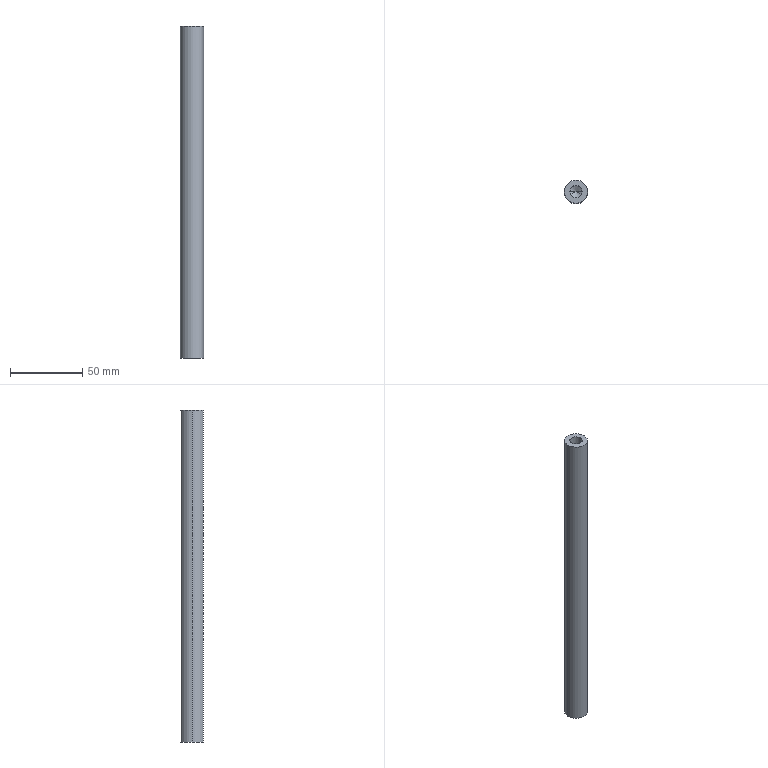Part | STEP file | B1-025 | 1 solid | 12 faces | box 16 x 16 x 230 mm | volume 44559 mm3 | cylinder 6 | cone 4 | plane 2 | commonest cylinder face diameters 8.5 x4 16 x2
STEP:
#1=CARTESIAN_POINT('',(0.,0.,0.));
#2=DIRECTION('',(0.,0.,1.));
#3=DIRECTION('',(1.,0.,0.));
#4=AXIS2_PLACEMENT_3D('',#1,#2,#3);
#5=CARTESIAN_POINT('',(4.25,0.,101.));
#6=VERTEX_POINT('',#5);
#7=CARTESIAN_POINT('',(4.25,0.,115.));
#8=VERTEX_POINT('',#7);
#9=CARTESIAN_POINT('',(4.25,0.,115.));
#10=DIRECTION('',(0.,0.,1.));
#11=VECTOR('',#10,1.);
#12=LINE('',#9,#11);
#13=CARTESIAN_POINT('',(0.,0.,115.));
#14=DIRECTION('',(0.,0.,1.));
#15=DIRECTION('',(1.,0.,0.));
#16=AXIS2_PLACEMENT_3D('',#13,#14,#15);
#17=CYLINDRICAL_SURFACE('',#16,4.25);
#18=CARTESIAN_POINT('',(6.283,0.));
#19=DIRECTION('',(0.,1.));
#20=VECTOR('',#19,1.);
#21=LINE('',#18,#20);
#22=(GEOMETRIC_REPRESENTATION_CONTEXT(2)PARAMETRIC_REPRESENTATION_CONTEXT()REPRESENTATION_CONTEXT('',''));
#23=DEFINITIONAL_REPRESENTATION('',(#21),#22);
#24=PCURVE('',#17,#23);
#25=CARTESIAN_POINT('',(0.,0.,115.));
#26=DIRECTION('',(0.,0.,1.));
#27=DIRECTION('',(1.,0.,0.));
#28=AXIS2_PLACEMENT_3D('',#25,#26,#27);
#29=CYLINDRICAL_SURFACE('',#28,4.25);
#30=CARTESIAN_POINT('',(0.,0.));
#31=DIRECTION('',(0.,1.));
#32=VECTOR('',#31,1.);
#33=LINE('',#30,#32);
#34=(GEOMETRIC_REPRESENTATION_CONTEXT(2)PARAMETRIC_REPRESENTATION_CONTEXT()REPRESENTATION_CONTEXT('',''));
#35=DEFINITIONAL_REPRESENTATION('',(#33),#34);
#36=PCURVE('',#29,#35);
#37=SURFACE_CURVE('',#12,(#24,#36),.PCURVE_S1.);
#38=EDGE_CURVE('',#6,#8,#37,.T.);
#39=ORIENTED_EDGE('',*,*,#38,.T.);
#40=CARTESIAN_POINT('',(-4.25,0.,115.));
#41=VERTEX_POINT('',#40);
#42=CARTESIAN_POINT('',(0.,0.,115.));
#43=DIRECTION('',(0.,0.,1.));
#44=DIRECTION('',(1.,0.,0.));
#45=AXIS2_PLACEMENT_3D('',#42,#43,#44);
#46=CIRCLE('',#45,4.25);
#47=CARTESIAN_POINT('',(0.,0.));
#48=DIRECTION('',(1.,0.));
#49=VECTOR('',#48,1.);
#50=LINE('',#47,#49);
#51=(GEOMETRIC_REPRESENTATION_CONTEXT(2)PARAMETRIC_REPRESENTATION_CONTEXT()REPRESENTATION_CONTEXT('',''));
#52=DEFINITIONAL_REPRESENTATION('',(#50),#51);
#53=PCURVE('',#17,#52);
#54=CARTESIAN_POINT('',(0.,0.,115.));
#55=DIRECTION('',(0.,0.,1.));
#56=DIRECTION('',(1.,0.,0.));
#57=AXIS2_PLACEMENT_3D('',#54,#55,#56);
#58=PLANE('',#57);
#59=CARTESIAN_POINT('',(0.,0.));
#60=DIRECTION('',(1.,0.));
#61=AXIS2_PLACEMENT_2D('',#59,#60);
#62=CIRCLE('',#61,4.25);
#63=(GEOMETRIC_REPRESENTATION_CONTEXT(2)PARAMETRIC_REPRESENTATION_CONTEXT()REPRESENTATION_CONTEXT('',''));
#64=DEFINITIONAL_REPRESENTATION('',(#62),#63);
#65=PCURVE('',#58,#64);
#66=SURFACE_CURVE('',#46,(#53,#65),.PCURVE_S1.);
#67=EDGE_CURVE('',#41,#8,#66,.T.);
#68=ORIENTED_EDGE('',*,*,#67,.F.);
#69=CARTESIAN_POINT('',(-4.25,0.,101.));
#70=VERTEX_POINT('',#69);
#71=CARTESIAN_POINT('',(-4.25,0.,115.));
#72=DIRECTION('',(0.,0.,1.));
#73=VECTOR('',#72,1.);
#74=LINE('',#71,#73);
#75=CARTESIAN_POINT('',(3.142,0.));
#76=DIRECTION('',(0.,1.));
#77=VECTOR('',#76,1.);
#78=LINE('',#75,#77);
#79=(GEOMETRIC_REPRESENTATION_CONTEXT(2)PARAMETRIC_REPRESENTATION_CONTEXT()REPRESENTATION_CONTEXT('',''));
#80=DEFINITIONAL_REPRESENTATION('',(#78),#79);
#81=PCURVE('',#17,#80);
#82=CARTESIAN_POINT('',(3.142,0.));
#83=DIRECTION('',(0.,1.));
#84=VECTOR('',#83,1.);
#85=LINE('',#82,#84);
#86=(GEOMETRIC_REPRESENTATION_CONTEXT(2)PARAMETRIC_REPRESENTATION_CONTEXT()REPRESENTATION_CONTEXT('',''));
#87=DEFINITIONAL_REPRESENTATION('',(#85),#86);
#88=PCURVE('',#29,#87);
#89=SURFACE_CURVE('',#74,(#81,#88),.PCURVE_S1.);
#90=EDGE_CURVE('',#70,#41,#89,.T.);
#91=ORIENTED_EDGE('',*,*,#90,.F.);
#92=CARTESIAN_POINT('',(0.,0.,101.));
#93=DIRECTION('',(0.,0.,1.));
#94=DIRECTION('',(1.,0.,0.));
#95=AXIS2_PLACEMENT_3D('',#92,#93,#94);
#96=CIRCLE('',#95,4.25);
#97=CARTESIAN_POINT('',(0.,-14.));
#98=DIRECTION('',(1.,0.));
#99=VECTOR('',#98,1.);
#100=LINE('',#97,#99);
#101=(GEOMETRIC_REPRESENTATION_CONTEXT(2)PARAMETRIC_REPRESENTATION_CONTEXT()REPRESENTATION_CONTEXT('',''));
#102=DEFINITIONAL_REPRESENTATION('',(#100),#101);
#103=PCURVE('',#17,#102);
#104=CARTESIAN_POINT('',(0.,0.,101.));
#105=DIRECTION('',(0.,0.,1.));
#106=DIRECTION('',(1.,0.,0.));
#107=AXIS2_PLACEMENT_3D('',#104,#105,#106);
#108=CONICAL_SURFACE('',#107,4.25,1.03);
#109=CARTESIAN_POINT('',(0.,0.));
#110=DIRECTION('',(1.,0.));
#111=VECTOR('',#110,1.);
#112=LINE('',#109,#111);
#113=(GEOMETRIC_REPRESENTATION_CONTEXT(2)PARAMETRIC_REPRESENTATION_CONTEXT()REPRESENTATION_CONTEXT('',''));
#114=DEFINITIONAL_REPRESENTATION('',(#112),#113);
#115=PCURVE('',#108,#114);
#116=SURFACE_CURVE('',#96,(#103,#115),.PCURVE_S1.);
#117=EDGE_CURVE('',#70,#6,#116,.T.);
#118=ORIENTED_EDGE('',*,*,#117,.T.);
#119=EDGE_LOOP('',(#39,#68,#91,#118));
#120=FACE_BOUND('',#119,.F.);
#121=ADVANCED_FACE('',(#120),#17,.F.);
#122=ORIENTED_EDGE('',*,*,#117,.F.);
#123=CARTESIAN_POINT('',(0.,0.,98.446));
#124=VERTEX_POINT('',#123);
#125=CARTESIAN_POINT('',(-4.25,0.,101.));
#126=DIRECTION('',(-0.8572,0.,0.515));
#127=VECTOR('',#126,1.);
#128=LINE('',#125,#127);
#129=CARTESIAN_POINT('',(3.142,0.));
#130=DIRECTION('',(0.,1.));
#131=VECTOR('',#130,1.);
#132=LINE('',#129,#131);
#133=(GEOMETRIC_REPRESENTATION_CONTEXT(2)PARAMETRIC_REPRESENTATION_CONTEXT()REPRESENTATION_CONTEXT('',''));
#134=DEFINITIONAL_REPRESENTATION('',(#132),#133);
#135=PCURVE('',#108,#134);
#136=CARTESIAN_POINT('',(0.,0.,101.));
#137=DIRECTION('',(0.,0.,1.));
#138=DIRECTION('',(1.,0.,0.));
#139=AXIS2_PLACEMENT_3D('',#136,#137,#138);
#140=CONICAL_SURFACE('',#139,4.25,1.03);
#141=CARTESIAN_POINT('',(3.142,0.));
#142=DIRECTION('',(0.,1.));
#143=VECTOR('',#142,1.);
#144=LINE('',#141,#143);
#145=(GEOMETRIC_REPRESENTATION_CONTEXT(2)PARAMETRIC_REPRESENTATION_CONTEXT()REPRESENTATION_CONTEXT('',''));
#146=DEFINITIONAL_REPRESENTATION('',(#144),#145);
#147=PCURVE('',#140,#146);
#148=SURFACE_CURVE('',#128,(#135,#147),.PCURVE_S1.);
#149=EDGE_CURVE('',#124,#70,#148,.T.);
#150=ORIENTED_EDGE('',*,*,#149,.F.);
#151=CARTESIAN_POINT('',(4.25,0.,101.));
#152=DIRECTION('',(0.8572,0.,0.515));
#153=VECTOR('',#152,1.);
#154=LINE('',#151,#153);
#155=CARTESIAN_POINT('',(6.283,-2.554));
#156=CARTESIAN_POINT('',(6.283,-2.515));
#157=CARTESIAN_POINT('',(6.283,-2.438));
#158=CARTESIAN_POINT('',(6.283,-2.322));
#159=CARTESIAN_POINT('',(6.283,-2.205));
#160=CARTESIAN_POINT('',(6.283,-2.089));
#161=CARTESIAN_POINT('',(6.283,-1.973));
#162=CARTESIAN_POINT('',(6.283,-1.857));
#163=CARTESIAN_POINT('',(6.283,-1.741));
#164=CARTESIAN_POINT('',(6.283,-1.625));
#165=CARTESIAN_POINT('',(6.283,-1.509));
#166=CARTESIAN_POINT('',(6.283,-1.393));
#167=CARTESIAN_POINT('',(6.283,-1.277));
#168=CARTESIAN_POINT('',(6.283,-1.161));
#169=CARTESIAN_POINT('',(6.283,-1.045));
#170=CARTESIAN_POINT('',(6.283,-0.9286));
#171=CARTESIAN_POINT('',(6.283,-0.8125));
#172=CARTESIAN_POINT('',(6.283,-0.6965));
#173=CARTESIAN_POINT('',(6.283,-0.5804));
#174=CARTESIAN_POINT('',(6.283,-0.4643));
#175=CARTESIAN_POINT('',(6.283,-0.3482));
#176=CARTESIAN_POINT('',(6.283,-0.2322));
#177=CARTESIAN_POINT('',(6.283,-0.1161));
#178=CARTESIAN_POINT('',(6.283,-0.03869));
#179=CARTESIAN_POINT('',(6.283,0.));
#180=B_SPLINE_CURVE_WITH_KNOTS('',3,(#155,#156,#157,#158,#159,#160,#161,#162,#163,#164,#165,#166,#167,#168,#169,#170,#171,#172,#173,#174,#175,#176,#177,#178,#179),.UNSPECIFIED.,.F.,.F.,(4,1,1,1,1,1,1,1,1,1,1,1,1,1,1,1,1,1,1,1,1,1,4),(-4.958,-4.733,-4.507,-4.282,-4.057,-3.831,-3.606,-3.381,-3.155,-2.93,-2.704,-2.479,-2.254,-2.028,-1.803,-1.578,-1.352,-1.127,-0.9015,-0.6761,-0.4507,-0.2254,0.),.QUASI_UNIFORM_KNOTS.);
#181=(GEOMETRIC_REPRESENTATION_CONTEXT(2)PARAMETRIC_REPRESENTATION_CONTEXT()REPRESENTATION_CONTEXT('',''));
#182=DEFINITIONAL_REPRESENTATION('',(#180),#181);
#183=PCURVE('',#108,#182);
#184=CARTESIAN_POINT('',(0.,-2.554));
#185=CARTESIAN_POINT('',(0.,-2.515));
#186=CARTESIAN_POINT('',(0.,-2.438));
#187=CARTESIAN_POINT('',(0.,-2.322));
#188=CARTESIAN_POINT('',(0.,-2.205));
#189=CARTESIAN_POINT('',(0.,-2.089));
#190=CARTESIAN_POINT('',(0.,-1.973));
#191=CARTESIAN_POINT('',(0.,-1.857));
#192=CARTESIAN_POINT('',(0.,-1.741));
#193=CARTESIAN_POINT('',(0.,-1.625));
#194=CARTESIAN_POINT('',(0.,-1.509));
#195=CARTESIAN_POINT('',(0.,-1.393));
#196=CARTESIAN_POINT('',(0.,-1.277));
#197=CARTESIAN_POINT('',(0.,-1.161));
#198=CARTESIAN_POINT('',(0.,-1.045));
#199=CARTESIAN_POINT('',(0.,-0.9286));
#200=CARTESIAN_POINT('',(0.,-0.8125));
#201=CARTESIAN_POINT('',(0.,-0.6965));
#202=CARTESIAN_POINT('',(0.,-0.5804));
#203=CARTESIAN_POINT('',(0.,-0.4643));
#204=CARTESIAN_POINT('',(0.,-0.3482));
#205=CARTESIAN_POINT('',(0.,-0.2322));
#206=CARTESIAN_POINT('',(0.,-0.1161));
#207=CARTESIAN_POINT('',(0.,-0.03869));
#208=CARTESIAN_POINT('',(0.,0.));
#209=B_SPLINE_CURVE_WITH_KNOTS('',3,(#184,#185,#186,#187,#188,#189,#190,#191,#192,#193,#194,#195,#196,#197,#198,#199,#200,#201,#202,#203,#204,#205,#206,#207,#208),.UNSPECIFIED.,.F.,.F.,(4,1,1,1,1,1,1,1,1,1,1,1,1,1,1,1,1,1,1,1,1,1,4),(-4.958,-4.733,-4.507,-4.282,-4.057,-3.831,-3.606,-3.381,-3.155,-2.93,-2.704,-2.479,-2.254,-2.028,-1.803,-1.578,-1.352,-1.127,-0.9015,-0.6761,-0.4507,-0.2254,0.),.QUASI_UNIFORM_KNOTS.);
#210=(GEOMETRIC_REPRESENTATION_CONTEXT(2)PARAMETRIC_REPRESENTATION_CONTEXT()REPRESENTATION_CONTEXT('',''));
#211=DEFINITIONAL_REPRESENTATION('',(#209),#210);
#212=PCURVE('',#140,#211);
#213=SURFACE_CURVE('',#154,(#183,#212),.PCURVE_S1.);
#214=EDGE_CURVE('',#124,#6,#213,.T.);
#215=ORIENTED_EDGE('',*,*,#214,.T.);
#216=EDGE_LOOP('',(#122,#150,#215));
#217=FACE_BOUND('',#216,.F.);
#218=ADVANCED_FACE('',(#217),#108,.F.);
#219=CARTESIAN_POINT('',(-4.25,0.,-101.));
#220=VERTEX_POINT('',#219);
#221=CARTESIAN_POINT('',(-4.25,0.,-115.));
#222=VERTEX_POINT('',#221);
#223=CARTESIAN_POINT('',(-4.25,0.,-115.));
#224=DIRECTION('',(0.,0.,-1.));
#225=VECTOR('',#224,1.);
#226=LINE('',#223,#225);
#227=CARTESIAN_POINT('',(0.,0.,-115.));
#228=DIRECTION('',(0.,0.,-1.));
#229=DIRECTION('',(-1.,0.,0.));
#230=AXIS2_PLACEMENT_3D('',#227,#228,#229);
#231=CYLINDRICAL_SURFACE('',#230,4.25);
#232=CARTESIAN_POINT('',(6.283,0.));
#233=DIRECTION('',(0.,1.));
#234=VECTOR('',#233,1.);
#235=LINE('',#232,#234);
#236=(GEOMETRIC_REPRESENTATION_CONTEXT(2)PARAMETRIC_REPRESENTATION_CONTEXT()REPRESENTATION_CONTEXT('',''));
#237=DEFINITIONAL_REPRESENTATION('',(#235),#236);
#238=PCURVE('',#231,#237);
#239=CARTESIAN_POINT('',(0.,0.,-115.));
#240=DIRECTION('',(0.,0.,-1.));
#241=DIRECTION('',(-1.,0.,0.));
#242=AXIS2_PLACEMENT_3D('',#239,#240,#241);
#243=CYLINDRICAL_SURFACE('',#242,4.25);
#244=CARTESIAN_POINT('',(0.,0.));
#245=DIRECTION('',(0.,1.));
#246=VECTOR('',#245,1.);
#247=LINE('',#244,#246);
#248=(GEOMETRIC_REPRESENTATION_CONTEXT(2)PARAMETRIC_REPRESENTATION_CONTEXT()REPRESENTATION_CONTEXT('',''));
#249=DEFINITIONAL_REPRESENTATION('',(#247),#248);
#250=PCURVE('',#243,#249);
#251=SURFACE_CURVE('',#226,(#238,#250),.PCURVE_S1.);
#252=EDGE_CURVE('',#220,#222,#251,.T.);
#253=ORIENTED_EDGE('',*,*,#252,.T.);
#254=CARTESIAN_POINT('',(4.25,0.,-115.));
#255=VERTEX_POINT('',#254);
#256=CARTESIAN_POINT('',(0.,0.,-115.));
#257=DIRECTION('',(0.,0.,-1.));
#258=DIRECTION('',(-1.,0.,0.));
#259=AXIS2_PLACEMENT_3D('',#256,#257,#258);
#260=CIRCLE('',#259,4.25);
#261=CARTESIAN_POINT('',(0.,0.));
#262=DIRECTION('',(1.,0.));
#263=VECTOR('',#262,1.);
#264=LINE('',#261,#263);
#265=(GEOMETRIC_REPRESENTATION_CONTEXT(2)PARAMETRIC_REPRESENTATION_CONTEXT()REPRESENTATION_CONTEXT('',''));
#266=DEFINITIONAL_REPRESENTATION('',(#264),#265);
#267=PCURVE('',#231,#266);
#268=CARTESIAN_POINT('',(0.,0.,-115.));
#269=DIRECTION('',(0.,0.,1.));
#270=DIRECTION('',(1.,0.,0.));
#271=AXIS2_PLACEMENT_3D('',#268,#269,#270);
#272=PLANE('',#271);
#273=CARTESIAN_POINT('',(-4.25,0.));
#274=CARTESIAN_POINT('',(-4.25,7.361));
#275=CARTESIAN_POINT('',(2.125,3.681));
#276=CARTESIAN_POINT('',(8.5,0.));
#277=CARTESIAN_POINT('',(2.125,-3.681));
#278=CARTESIAN_POINT('',(-4.25,-7.361));
#279=CARTESIAN_POINT('',(-4.25,0.));
#280=(BOUNDED_CURVE()B_SPLINE_CURVE(2,(#273,#274,#275,#276,#277,#278,#279),.UNSPECIFIED.,.T.,.F.)B_SPLINE_CURVE_WITH_KNOTS((1,2,2,2,2,1),(-2.094,0.,2.094,4.189,6.283,8.378),.UNSPECIFIED.)CURVE()GEOMETRIC_REPRESENTATION_ITEM()RATIONAL_B_SPLINE_CURVE((1.,0.5,1.,0.5,1.,0.5,1.))REPRESENTATION_ITEM(''));
#281=(GEOMETRIC_REPRESENTATION_CONTEXT(2)PARAMETRIC_REPRESENTATION_CONTEXT()REPRESENTATION_CONTEXT('',''));
#282=DEFINITIONAL_REPRESENTATION('',(#280),#281);
#283=PCURVE('',#272,#282);
#284=SURFACE_CURVE('',#260,(#267,#283),.PCURVE_S1.);
#285=EDGE_CURVE('',#255,#222,#284,.T.);
#286=ORIENTED_EDGE('',*,*,#285,.F.);
#287=CARTESIAN_POINT('',(4.25,0.,-101.));
#288=VERTEX_POINT('',#287);
#289=CARTESIAN_POINT('',(4.25,0.,-115.));
#290=DIRECTION('',(0.,0.,-1.));
#291=VECTOR('',#290,1.);
#292=LINE('',#289,#291);
#293=CARTESIAN_POINT('',(3.142,0.));
#294=DIRECTION('',(0.,1.));
#295=VECTOR('',#294,1.);
#296=LINE('',#293,#295);
#297=(GEOMETRIC_REPRESENTATION_CONTEXT(2)PARAMETRIC_REPRESENTATION_CONTEXT()REPRESENTATION_CONTEXT('',''));
#298=DEFINITIONAL_REPRESENTATION('',(#296),#297);
#299=PCURVE('',#231,#298);
#300=CARTESIAN_POINT('',(3.142,0.));
#301=DIRECTION('',(0.,1.));
#302=VECTOR('',#301,1.);
#303=LINE('',#300,#302);
#304=(GEOMETRIC_REPRESENTATION_CONTEXT(2)PARAMETRIC_REPRESENTATION_CONTEXT()REPRESENTATION_CONTEXT('',''));
#305=DEFINITIONAL_REPRESENTATION('',(#303),#304);
#306=PCURVE('',#243,#305);
#307=SURFACE_CURVE('',#292,(#299,#306),.PCURVE_S1.);
#308=EDGE_CURVE('',#288,#255,#307,.T.);
#309=ORIENTED_EDGE('',*,*,#308,.F.);
#310=CARTESIAN_POINT('',(0.,0.,-101.));
#311=DIRECTION('',(0.,0.,-1.));
#312=DIRECTION('',(-1.,0.,0.));
#313=AXIS2_PLACEMENT_3D('',#310,#311,#312);
#314=CIRCLE('',#313,4.25);
#315=CARTESIAN_POINT('',(0.,-14.));
#316=DIRECTION('',(1.,0.));
#317=VECTOR('',#316,1.);
#318=LINE('',#315,#317);
#319=(GEOMETRIC_REPRESENTATION_CONTEXT(2)PARAMETRIC_REPRESENTATION_CONTEXT()REPRESENTATION_CONTEXT('',''));
#320=DEFINITIONAL_REPRESENTATION('',(#318),#319);
#321=PCURVE('',#231,#320);
#322=CARTESIAN_POINT('',(0.,0.,-101.));
#323=DIRECTION('',(0.,0.,-1.));
#324=DIRECTION('',(-1.,0.,0.));
#325=AXIS2_PLACEMENT_3D('',#322,#323,#324);
#326=CONICAL_SURFACE('',#325,4.25,1.03);
#327=CARTESIAN_POINT('',(0.,0.));
#328=DIRECTION('',(1.,0.));
#329=VECTOR('',#328,1.);
#330=LINE('',#327,#329);
#331=(GEOMETRIC_REPRESENTATION_CONTEXT(2)PARAMETRIC_REPRESENTATION_CONTEXT()REPRESENTATION_CONTEXT('',''));
#332=DEFINITIONAL_REPRESENTATION('',(#330),#331);
#333=PCURVE('',#326,#332);
#334=SURFACE_CURVE('',#314,(#321,#333),.PCURVE_S1.);
#335=EDGE_CURVE('',#288,#220,#334,.T.);
#336=ORIENTED_EDGE('',*,*,#335,.T.);
#337=EDGE_LOOP('',(#253,#286,#309,#336));
#338=FACE_BOUND('',#337,.F.);
#339=ADVANCED_FACE('',(#338),#231,.F.);
#340=ORIENTED_EDGE('',*,*,#335,.F.);
#341=CARTESIAN_POINT('',(0.,0.,-98.446));
#342=VERTEX_POINT('',#341);
#343=CARTESIAN_POINT('',(4.25,0.,-101.));
#344=DIRECTION('',(0.8572,0.,-0.515));
#345=VECTOR('',#344,1.);
#346=LINE('',#343,#345);
#347=CARTESIAN_POINT('',(3.142,-2.554));
#348=CARTESIAN_POINT('',(3.142,-2.515));
#349=CARTESIAN_POINT('',(3.142,-2.438));
#350=CARTESIAN_POINT('',(3.142,-2.322));
#351=CARTESIAN_POINT('',(3.142,-2.205));
#352=CARTESIAN_POINT('',(3.142,-2.089));
#353=CARTESIAN_POINT('',(3.142,-1.973));
#354=CARTESIAN_POINT('',(3.142,-1.857));
#355=CARTESIAN_POINT('',(3.142,-1.741));
#356=CARTESIAN_POINT('',(3.142,-1.625));
#357=CARTESIAN_POINT('',(3.142,-1.509));
#358=CARTESIAN_POINT('',(3.142,-1.393));
#359=CARTESIAN_POINT('',(3.142,-1.277));
#360=CARTESIAN_POINT('',(3.142,-1.161));
#361=CARTESIAN_POINT('',(3.142,-1.045));
#362=CARTESIAN_POINT('',(3.142,-0.9286));
#363=CARTESIAN_POINT('',(3.142,-0.8125));
#364=CARTESIAN_POINT('',(3.142,-0.6965));
#365=CARTESIAN_POINT('',(3.142,-0.5804));
#366=CARTESIAN_POINT('',(3.142,-0.4643));
#367=CARTESIAN_POINT('',(3.142,-0.3482));
#368=CARTESIAN_POINT('',(3.142,-0.2322));
#369=CARTESIAN_POINT('',(3.142,-0.1161));
#370=CARTESIAN_POINT('',(3.142,-0.03869));
#371=CARTESIAN_POINT('',(3.142,0.));
#372=B_SPLINE_CURVE_WITH_KNOTS('',3,(#347,#348,#349,#350,#351,#352,#353,#354,#355,#356,#357,#358,#359,#360,#361,#362,#363,#364,#365,#366,#367,#368,#369,#370,#371),.UNSPECIFIED.,.F.,.F.,(4,1,1,1,1,1,1,1,1,1,1,1,1,1,1,1,1,1,1,1,1,1,4),(-4.958,-4.733,-4.507,-4.282,-4.057,-3.831,-3.606,-3.381,-3.155,-2.93,-2.704,-2.479,-2.254,-2.028,-1.803,-1.578,-1.352,-1.127,-0.9015,-0.6761,-0.4507,-0.2254,0.),.QUASI_UNIFORM_KNOTS.);
#373=(GEOMETRIC_REPRESENTATION_CONTEXT(2)PARAMETRIC_REPRESENTATION_CONTEXT()REPRESENTATION_CONTEXT('',''));
#374=DEFINITIONAL_REPRESENTATION('',(#372),#373);
#375=PCURVE('',#326,#374);
#376=CARTESIAN_POINT('',(0.,0.,-101.));
#377=DIRECTION('',(0.,0.,-1.));
#378=DIRECTION('',(-1.,0.,0.));
#379=AXIS2_PLACEMENT_3D('',#376,#377,#378);
#380=CONICAL_SURFACE('',#379,4.25,1.03);
#381=CARTESIAN_POINT('',(3.142,-2.554));
#382=CARTESIAN_POINT('',(3.142,-2.515));
#383=CARTESIAN_POINT('',(3.142,-2.438));
#384=CARTESIAN_POINT('',(3.142,-2.322));
#385=CARTESIAN_POINT('',(3.142,-2.205));
#386=CARTESIAN_POINT('',(3.142,-2.089));
#387=CARTESIAN_POINT('',(3.142,-1.973));
#388=CARTESIAN_POINT('',(3.142,-1.857));
#389=CARTESIAN_POINT('',(3.142,-1.741));
#390=CARTESIAN_POINT('',(3.142,-1.625));
#391=CARTESIAN_POINT('',(3.142,-1.509));
#392=CARTESIAN_POINT('',(3.142,-1.393));
#393=CARTESIAN_POINT('',(3.142,-1.277));
#394=CARTESIAN_POINT('',(3.142,-1.161));
#395=CARTESIAN_POINT('',(3.142,-1.045));
#396=CARTESIAN_POINT('',(3.142,-0.9286));
#397=CARTESIAN_POINT('',(3.142,-0.8125));
#398=CARTESIAN_POINT('',(3.142,-0.6965));
#399=CARTESIAN_POINT('',(3.142,-0.5804));
#400=CARTESIAN_POINT('',(3.142,-0.4643));
#401=CARTESIAN_POINT('',(3.142,-0.3482));
#402=CARTESIAN_POINT('',(3.142,-0.2322));
#403=CARTESIAN_POINT('',(3.142,-0.1161));
#404=CARTESIAN_POINT('',(3.142,-0.03869));
#405=CARTESIAN_POINT('',(3.142,0.));
#406=B_SPLINE_CURVE_WITH_KNOTS('',3,(#381,#382,#383,#384,#385,#386,#387,#388,#389,#390,#391,#392,#393,#394,#395,#396,#397,#398,#399,#400,#401,#402,#403,#404,#405),.UNSPECIFIED.,.F.,.F.,(4,1,1,1,1,1,1,1,1,1,1,1,1,1,1,1,1,1,1,1,1,1,4),(-4.958,-4.733,-4.507,-4.282,-4.057,-3.831,-3.606,-3.381,-3.155,-2.93,-2.704,-2.479,-2.254,-2.028,-1.803,-1.578,-1.352,-1.127,-0.9015,-0.6761,-0.4507,-0.2254,0.),.QUASI_UNIFORM_KNOTS.);
#407=(GEOMETRIC_REPRESENTATION_CONTEXT(2)PARAMETRIC_REPRESENTATION_CONTEXT()REPRESENTATION_CONTEXT('',''));
#408=DEFINITIONAL_REPRESENTATION('',(#406),#407);
#409=PCURVE('',#380,#408);
#410=SURFACE_CURVE('',#346,(#375,#409),.PCURVE_S1.);
#411=EDGE_CURVE('',#342,#288,#410,.T.);
#412=ORIENTED_EDGE('',*,*,#411,.F.);
#413=CARTESIAN_POINT('',(-4.25,0.,-101.));
#414=DIRECTION('',(-0.8572,0.,-0.515));
#415=VECTOR('',#414,1.);
#416=LINE('',#413,#415);
#417=CARTESIAN_POINT('',(6.283,0.));
#418=DIRECTION('',(0.,1.));
#419=VECTOR('',#418,1.);
#420=LINE('',#417,#419);
#421=(GEOMETRIC_REPRESENTATION_CONTEXT(2)PARAMETRIC_REPRESENTATION_CONTEXT()REPRESENTATION_CONTEXT('',''));
#422=DEFINITIONAL_REPRESENTATION('',(#420),#421);
#423=PCURVE('',#326,#422);
#424=CARTESIAN_POINT('',(0.,0.));
#425=DIRECTION('',(0.,1.));
#426=VECTOR('',#425,1.);
#427=LINE('',#424,#426);
#428=(GEOMETRIC_REPRESENTATION_CONTEXT(2)PARAMETRIC_REPRESENTATION_CONTEXT()REPRESENTATION_CONTEXT('',''));
#429=DEFINITIONAL_REPRESENTATION('',(#427),#428);
#430=PCURVE('',#380,#429);
#431=SURFACE_CURVE('',#416,(#423,#430),.PCURVE_S1.);
#432=EDGE_CURVE('',#342,#220,#431,.T.);
#433=ORIENTED_EDGE('',*,*,#432,.T.);
#434=EDGE_LOOP('',(#340,#412,#433));
#435=FACE_BOUND('',#434,.F.);
#436=ADVANCED_FACE('',(#435),#326,.F.);
#437=CARTESIAN_POINT('',(8.,0.,115.));
#438=VERTEX_POINT('',#437);
#439=CARTESIAN_POINT('',(-8.,0.,115.));
#440=VERTEX_POINT('',#439);
#441=CARTESIAN_POINT('',(0.,0.,115.));
#442=DIRECTION('',(0.,0.,1.));
#443=DIRECTION('',(1.,0.,0.));
#444=AXIS2_PLACEMENT_3D('',#441,#442,#443);
#445=CIRCLE('',#444,8.);
#446=CARTESIAN_POINT('',(0.,0.,115.));
#447=DIRECTION('',(0.,0.,-1.));
#448=DIRECTION('',(-1.,0.,0.));
#449=AXIS2_PLACEMENT_3D('',#446,#447,#448);
#450=CYLINDRICAL_SURFACE('',#449,8.);
#451=CARTESIAN_POINT('',(3.142,0.));
#452=DIRECTION('',(-1.,0.));
#453=VECTOR('',#452,1.);
#454=LINE('',#451,#453);
#455=(GEOMETRIC_REPRESENTATION_CONTEXT(2)PARAMETRIC_REPRESENTATION_CONTEXT()REPRESENTATION_CONTEXT('',''));
#456=DEFINITIONAL_REPRESENTATION('',(#454),#455);
#457=PCURVE('',#450,#456);
#458=CARTESIAN_POINT('',(0.,0.));
#459=DIRECTION('',(1.,0.));
#460=AXIS2_PLACEMENT_2D('',#458,#459);
#461=CIRCLE('',#460,8.);
#462=(GEOMETRIC_REPRESENTATION_CONTEXT(2)PARAMETRIC_REPRESENTATION_CONTEXT()REPRESENTATION_CONTEXT('',''));
#463=DEFINITIONAL_REPRESENTATION('',(#461),#462);
#464=PCURVE('',#58,#463);
#465=SURFACE_CURVE('',#445,(#457,#464),.PCURVE_S1.);
#466=EDGE_CURVE('',#438,#440,#465,.T.);
#467=ORIENTED_EDGE('',*,*,#466,.F.);
#468=CARTESIAN_POINT('',(8.,0.,-115.));
#469=VERTEX_POINT('',#468);
#470=CARTESIAN_POINT('',(8.,0.,115.));
#471=DIRECTION('',(0.,0.,-1.));
#472=VECTOR('',#471,1.);
#473=LINE('',#470,#472);
#474=CARTESIAN_POINT('',(3.142,0.));
#475=DIRECTION('',(0.,1.));
#476=VECTOR('',#475,1.);
#477=LINE('',#474,#476);
#478=(GEOMETRIC_REPRESENTATION_CONTEXT(2)PARAMETRIC_REPRESENTATION_CONTEXT()REPRESENTATION_CONTEXT('',''));
#479=DEFINITIONAL_REPRESENTATION('',(#477),#478);
#480=PCURVE('',#450,#479);
#481=CARTESIAN_POINT('',(0.,0.,115.));
#482=DIRECTION('',(0.,0.,-1.));
#483=DIRECTION('',(-1.,0.,0.));
#484=AXIS2_PLACEMENT_3D('',#481,#482,#483);
#485=CYLINDRICAL_SURFACE('',#484,8.);
#486=CARTESIAN_POINT('',(3.142,0.));
#487=DIRECTION('',(0.,1.));
#488=VECTOR('',#487,1.);
#489=LINE('',#486,#488);
#490=(GEOMETRIC_REPRESENTATION_CONTEXT(2)PARAMETRIC_REPRESENTATION_CONTEXT()REPRESENTATION_CONTEXT('',''));
#491=DEFINITIONAL_REPRESENTATION('',(#489),#490);
#492=PCURVE('',#485,#491);
#493=SURFACE_CURVE('',#473,(#480,#492),.PCURVE_S1.);
#494=EDGE_CURVE('',#438,#469,#493,.T.);
#495=ORIENTED_EDGE('',*,*,#494,.T.);
#496=CARTESIAN_POINT('',(-8.,0.,-115.));
#497=VERTEX_POINT('',#496);
#498=CARTESIAN_POINT('',(0.,0.,-115.));
#499=DIRECTION('',(0.,0.,1.));
#500=DIRECTION('',(1.,0.,0.));
#501=AXIS2_PLACEMENT_3D('',#498,#499,#500);
#502=CIRCLE('',#501,8.);
#503=CARTESIAN_POINT('',(3.142,230.));
#504=DIRECTION('',(-1.,0.));
#505=VECTOR('',#504,1.);
#506=LINE('',#503,#505);
#507=(GEOMETRIC_REPRESENTATION_CONTEXT(2)PARAMETRIC_REPRESENTATION_CONTEXT()REPRESENTATION_CONTEXT('',''));
#508=DEFINITIONAL_REPRESENTATION('',(#506),#507);
#509=PCURVE('',#450,#508);
#510=CARTESIAN_POINT('',(0.,0.));
#511=DIRECTION('',(1.,0.));
#512=AXIS2_PLACEMENT_2D('',#510,#511);
#513=CIRCLE('',#512,8.);
#514=(GEOMETRIC_REPRESENTATION_CONTEXT(2)PARAMETRIC_REPRESENTATION_CONTEXT()REPRESENTATION_CONTEXT('',''));
#515=DEFINITIONAL_REPRESENTATION('',(#513),#514);
#516=PCURVE('',#272,#515);
#517=SURFACE_CURVE('',#502,(#509,#516),.PCURVE_S1.);
#518=EDGE_CURVE('',#469,#497,#517,.T.);
#519=ORIENTED_EDGE('',*,*,#518,.T.);
#520=CARTESIAN_POINT('',(-8.,0.,115.));
#521=DIRECTION('',(0.,0.,-1.));
#522=VECTOR('',#521,1.);
#523=LINE('',#520,#522);
#524=CARTESIAN_POINT('',(0.,0.));
#525=DIRECTION('',(0.,1.));
#526=VECTOR('',#525,1.);
#527=LINE('',#524,#526);
#528=(GEOMETRIC_REPRESENTATION_CONTEXT(2)PARAMETRIC_REPRESENTATION_CONTEXT()REPRESENTATION_CONTEXT('',''));
#529=DEFINITIONAL_REPRESENTATION('',(#527),#528);
#530=PCURVE('',#450,#529);
#531=CARTESIAN_POINT('',(6.283,0.));
#532=DIRECTION('',(0.,1.));
#533=VECTOR('',#532,1.);
#534=LINE('',#531,#533);
#535=(GEOMETRIC_REPRESENTATION_CONTEXT(2)PARAMETRIC_REPRESENTATION_CONTEXT()REPRESENTATION_CONTEXT('',''));
#536=DEFINITIONAL_REPRESENTATION('',(#534),#535);
#537=PCURVE('',#485,#536);
#538=SURFACE_CURVE('',#523,(#530,#537),.PCURVE_S1.);
#539=EDGE_CURVE('',#440,#497,#538,.T.);
#540=ORIENTED_EDGE('',*,*,#539,.F.);
#541=EDGE_LOOP('',(#467,#495,#519,#540));
#542=FACE_BOUND('',#541,.T.);
#543=ADVANCED_FACE('',(#542),#450,.T.);
#544=CARTESIAN_POINT('',(0.,0.,-115.));
#545=DIRECTION('',(0.,0.,1.));
#546=DIRECTION('',(1.,0.,0.));
#547=AXIS2_PLACEMENT_3D('',#544,#545,#546);
#548=CIRCLE('',#547,8.);
#549=CARTESIAN_POINT('',(0.,0.));
#550=DIRECTION('',(1.,0.));
#551=AXIS2_PLACEMENT_2D('',#549,#550);
#552=CIRCLE('',#551,8.);
#553=(GEOMETRIC_REPRESENTATION_CONTEXT(2)PARAMETRIC_REPRESENTATION_CONTEXT()REPRESENTATION_CONTEXT('',''));
#554=DEFINITIONAL_REPRESENTATION('',(#552),#553);
#555=PCURVE('',#272,#554);
#556=CARTESIAN_POINT('',(9.425,230.));
#557=DIRECTION('',(-1.,0.));
#558=VECTOR('',#557,1.);
#559=LINE('',#556,#558);
#560=(GEOMETRIC_REPRESENTATION_CONTEXT(2)PARAMETRIC_REPRESENTATION_CONTEXT()REPRESENTATION_CONTEXT('',''));
#561=DEFINITIONAL_REPRESENTATION('',(#559),#560);
#562=PCURVE('',#485,#561);
#563=SURFACE_CURVE('',#548,(#555,#562),.PCURVE_S1.);
#564=EDGE_CURVE('',#497,#469,#563,.T.);
#565=ORIENTED_EDGE('',*,*,#564,.F.);
#566=ORIENTED_EDGE('',*,*,#518,.F.);
#567=EDGE_LOOP('',(#565,#566));
#568=FACE_BOUND('',#567,.T.);
#569=CARTESIAN_POINT('',(0.,0.,-115.));
#570=DIRECTION('',(0.,0.,-1.));
#571=DIRECTION('',(-1.,0.,0.));
#572=AXIS2_PLACEMENT_3D('',#569,#570,#571);
#573=CIRCLE('',#572,4.25);
#574=CARTESIAN_POINT('',(-4.25,0.));
#575=CARTESIAN_POINT('',(-4.25,7.361));
#576=CARTESIAN_POINT('',(2.125,3.681));
#577=CARTESIAN_POINT('',(8.5,0.));
#578=CARTESIAN_POINT('',(2.125,-3.681));
#579=CARTESIAN_POINT('',(-4.25,-7.361));
#580=CARTESIAN_POINT('',(-4.25,0.));
#581=(BOUNDED_CURVE()B_SPLINE_CURVE(2,(#574,#575,#576,#577,#578,#579,#580),.UNSPECIFIED.,.T.,.F.)B_SPLINE_CURVE_WITH_KNOTS((1,2,2,2,2,1),(-2.094,0.,2.094,4.189,6.283,8.378),.UNSPECIFIED.)CURVE()GEOMETRIC_REPRESENTATION_ITEM()RATIONAL_B_SPLINE_CURVE((1.,0.5,1.,0.5,1.,0.5,1.))REPRESENTATION_ITEM(''));
#582=(GEOMETRIC_REPRESENTATION_CONTEXT(2)PARAMETRIC_REPRESENTATION_CONTEXT()REPRESENTATION_CONTEXT('',''));
#583=DEFINITIONAL_REPRESENTATION('',(#581),#582);
#584=PCURVE('',#272,#583);
#585=CARTESIAN_POINT('',(0.,0.));
#586=DIRECTION('',(1.,0.));
#587=VECTOR('',#586,1.);
#588=LINE('',#585,#587);
#589=(GEOMETRIC_REPRESENTATION_CONTEXT(2)PARAMETRIC_REPRESENTATION_CONTEXT()REPRESENTATION_CONTEXT('',''));
#590=DEFINITIONAL_REPRESENTATION('',(#588),#589);
#591=PCURVE('',#243,#590);
#592=SURFACE_CURVE('',#573,(#584,#591),.PCURVE_S1.);
#593=EDGE_CURVE('',#222,#255,#592,.T.);
#594=ORIENTED_EDGE('',*,*,#593,.F.);
#595=ORIENTED_EDGE('',*,*,#285,.F.);
#596=EDGE_LOOP('',(#594,#595));
#597=FACE_BOUND('',#596,.T.);
#598=ADVANCED_FACE('',(#568,#597),#272,.F.);
#599=ORIENTED_EDGE('',*,*,#494,.F.);
#600=CARTESIAN_POINT('',(0.,0.,115.));
#601=DIRECTION('',(0.,0.,1.));
#602=DIRECTION('',(1.,0.,0.));
#603=AXIS2_PLACEMENT_3D('',#600,#601,#602);
#604=CIRCLE('',#603,8.);
#605=CARTESIAN_POINT('',(9.425,0.));
#606=DIRECTION('',(-1.,0.));
#607=VECTOR('',#606,1.);
#608=LINE('',#605,#607);
#609=(GEOMETRIC_REPRESENTATION_CONTEXT(2)PARAMETRIC_REPRESENTATION_CONTEXT()REPRESENTATION_CONTEXT('',''));
#610=DEFINITIONAL_REPRESENTATION('',(#608),#609);
#611=PCURVE('',#485,#610);
#612=CARTESIAN_POINT('',(0.,0.));
#613=DIRECTION('',(1.,0.));
#614=AXIS2_PLACEMENT_2D('',#612,#613);
#615=CIRCLE('',#614,8.);
#616=(GEOMETRIC_REPRESENTATION_CONTEXT(2)PARAMETRIC_REPRESENTATION_CONTEXT()REPRESENTATION_CONTEXT('',''));
#617=DEFINITIONAL_REPRESENTATION('',(#615),#616);
#618=PCURVE('',#58,#617);
#619=SURFACE_CURVE('',#604,(#611,#618),.PCURVE_S1.);
#620=EDGE_CURVE('',#440,#438,#619,.T.);
#621=ORIENTED_EDGE('',*,*,#620,.F.);
#622=ORIENTED_EDGE('',*,*,#539,.T.);
#623=ORIENTED_EDGE('',*,*,#564,.T.);
#624=EDGE_LOOP('',(#599,#621,#622,#623));
#625=FACE_BOUND('',#624,.T.);
#626=ADVANCED_FACE('',(#625),#485,.T.);
#627=CARTESIAN_POINT('',(0.,0.,115.));
#628=DIRECTION('',(0.,0.,1.));
#629=DIRECTION('',(1.,0.,0.));
#630=AXIS2_PLACEMENT_3D('',#627,#628,#629);
#631=CIRCLE('',#630,4.25);
#632=CARTESIAN_POINT('',(0.,0.));
#633=DIRECTION('',(1.,0.));
#634=AXIS2_PLACEMENT_2D('',#632,#633);
#635=CIRCLE('',#634,4.25);
#636=(GEOMETRIC_REPRESENTATION_CONTEXT(2)PARAMETRIC_REPRESENTATION_CONTEXT()REPRESENTATION_CONTEXT('',''));
#637=DEFINITIONAL_REPRESENTATION('',(#635),#636);
#638=PCURVE('',#58,#637);
#639=CARTESIAN_POINT('',(0.,0.));
#640=DIRECTION('',(1.,0.));
#641=VECTOR('',#640,1.);
#642=LINE('',#639,#641);
#643=(GEOMETRIC_REPRESENTATION_CONTEXT(2)PARAMETRIC_REPRESENTATION_CONTEXT()REPRESENTATION_CONTEXT('',''));
#644=DEFINITIONAL_REPRESENTATION('',(#642),#643);
#645=PCURVE('',#29,#644);
#646=SURFACE_CURVE('',#631,(#638,#645),.PCURVE_S1.);
#647=EDGE_CURVE('',#8,#41,#646,.T.);
#648=ORIENTED_EDGE('',*,*,#647,.F.);
#649=ORIENTED_EDGE('',*,*,#67,.F.);
#650=EDGE_LOOP('',(#648,#649));
#651=FACE_BOUND('',#650,.T.);
#652=ORIENTED_EDGE('',*,*,#620,.T.);
#653=ORIENTED_EDGE('',*,*,#466,.T.);
#654=EDGE_LOOP('',(#652,#653));
#655=FACE_BOUND('',#654,.T.);
#656=ADVANCED_FACE('',(#651,#655),#58,.T.);
#657=CARTESIAN_POINT('',(0.,0.,-101.));
#658=DIRECTION('',(0.,0.,-1.));
#659=DIRECTION('',(-1.,0.,0.));
#660=AXIS2_PLACEMENT_3D('',#657,#658,#659);
#661=CIRCLE('',#660,4.25);
#662=CARTESIAN_POINT('',(0.,0.));
#663=DIRECTION('',(1.,0.));
#664=VECTOR('',#663,1.);
#665=LINE('',#662,#664);
#666=(GEOMETRIC_REPRESENTATION_CONTEXT(2)PARAMETRIC_REPRESENTATION_CONTEXT()REPRESENTATION_CONTEXT('',''));
#667=DEFINITIONAL_REPRESENTATION('',(#665),#666);
#668=PCURVE('',#380,#667);
#669=CARTESIAN_POINT('',(0.,-14.));
#670=DIRECTION('',(1.,0.));
#671=VECTOR('',#670,1.);
#672=LINE('',#669,#671);
#673=(GEOMETRIC_REPRESENTATION_CONTEXT(2)PARAMETRIC_REPRESENTATION_CONTEXT()REPRESENTATION_CONTEXT('',''));
#674=DEFINITIONAL_REPRESENTATION('',(#672),#673);
#675=PCURVE('',#243,#674);
#676=SURFACE_CURVE('',#661,(#668,#675),.PCURVE_S1.);
#677=EDGE_CURVE('',#220,#288,#676,.T.);
#678=ORIENTED_EDGE('',*,*,#677,.F.);
#679=ORIENTED_EDGE('',*,*,#432,.F.);
#680=ORIENTED_EDGE('',*,*,#411,.T.);
#681=EDGE_LOOP('',(#678,#679,#680));
#682=FACE_BOUND('',#681,.F.);
#683=ADVANCED_FACE('',(#682),#380,.F.);
#684=ORIENTED_EDGE('',*,*,#593,.F.);
#685=ORIENTED_EDGE('',*,*,#252,.F.);
#686=ORIENTED_EDGE('',*,*,#677,.T.);
#687=ORIENTED_EDGE('',*,*,#308,.T.);
#688=EDGE_LOOP('',(#684,#685,#686,#687));
#689=FACE_BOUND('',#688,.F.);
#690=ADVANCED_FACE('',(#689),#243,.F.);
#691=CARTESIAN_POINT('',(0.,0.,101.));
#692=DIRECTION('',(0.,0.,1.));
#693=DIRECTION('',(1.,0.,0.));
#694=AXIS2_PLACEMENT_3D('',#691,#692,#693);
#695=CIRCLE('',#694,4.25);
#696=CARTESIAN_POINT('',(0.,0.));
#697=DIRECTION('',(1.,0.));
#698=VECTOR('',#697,1.);
#699=LINE('',#696,#698);
#700=(GEOMETRIC_REPRESENTATION_CONTEXT(2)PARAMETRIC_REPRESENTATION_CONTEXT()REPRESENTATION_CONTEXT('',''));
#701=DEFINITIONAL_REPRESENTATION('',(#699),#700);
#702=PCURVE('',#140,#701);
#703=CARTESIAN_POINT('',(0.,-14.));
#704=DIRECTION('',(1.,0.));
#705=VECTOR('',#704,1.);
#706=LINE('',#703,#705);
#707=(GEOMETRIC_REPRESENTATION_CONTEXT(2)PARAMETRIC_REPRESENTATION_CONTEXT()REPRESENTATION_CONTEXT('',''));
#708=DEFINITIONAL_REPRESENTATION('',(#706),#707);
#709=PCURVE('',#29,#708);
#710=SURFACE_CURVE('',#695,(#702,#709),.PCURVE_S1.);
#711=EDGE_CURVE('',#6,#70,#710,.T.);
#712=ORIENTED_EDGE('',*,*,#711,.F.);
#713=ORIENTED_EDGE('',*,*,#214,.F.);
#714=ORIENTED_EDGE('',*,*,#149,.T.);
#715=EDGE_LOOP('',(#712,#713,#714));
#716=FACE_BOUND('',#715,.F.);
#717=ADVANCED_FACE('',(#716),#140,.F.);
#718=ORIENTED_EDGE('',*,*,#647,.F.);
#719=ORIENTED_EDGE('',*,*,#38,.F.);
#720=ORIENTED_EDGE('',*,*,#711,.T.);
#721=ORIENTED_EDGE('',*,*,#90,.T.);
#722=EDGE_LOOP('',(#718,#719,#720,#721));
#723=FACE_BOUND('',#722,.F.);
#724=ADVANCED_FACE('',(#723),#29,.F.);
#725=CLOSED_SHELL('',(#121,#218,#339,#436,#543,#598,#626,#656,#683,#690,#717,#724));
#726=MANIFOLD_SOLID_BREP('',#725);
#727=(LENGTH_UNIT()NAMED_UNIT(*)SI_UNIT(.MILLI.,.METRE.));
#728=UNCERTAINTY_MEASURE_WITH_UNIT(LENGTH_MEASURE(0.0000001),#727,'','');
#729=(NAMED_UNIT(*)PLANE_ANGLE_UNIT()SI_UNIT($,.RADIAN.));
#730=(NAMED_UNIT(*)SI_UNIT($,.STERADIAN.)SOLID_ANGLE_UNIT());
#731=(GEOMETRIC_REPRESENTATION_CONTEXT(3)GLOBAL_UNCERTAINTY_ASSIGNED_CONTEXT((#728))GLOBAL_UNIT_ASSIGNED_CONTEXT((#727,#729,#730))REPRESENTATION_CONTEXT('',''));
#732=ADVANCED_BREP_SHAPE_REPRESENTATION('',(#4,#726),#731);